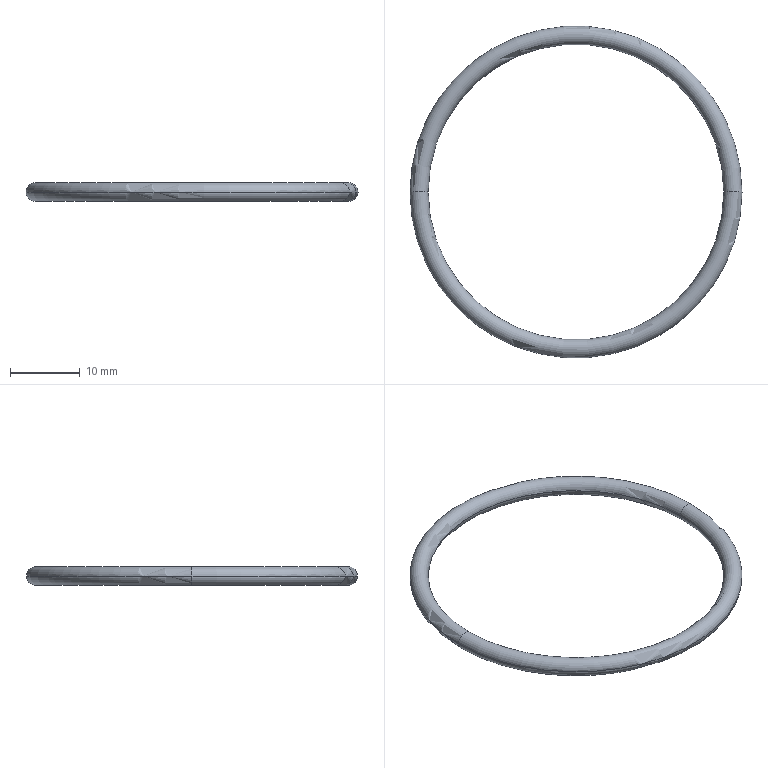Part | NX | features REVOLVE1 2 | 1 solid | 4 faces | box 47.752 x 47.752 x 2.616 mm | volume 762.259 mm3 | torus 4
STEP:
#1=CARTESIAN_POINT('',(-23.876,0.,0.));
#2=VERTEX_POINT('',#1);
#3=CARTESIAN_POINT('',(-21.26,0.,0.));
#4=VERTEX_POINT('',#3);
#5=CARTESIAN_POINT('',(-22.568,0.,0.));
#6=DIRECTION('',(0.,1.,0.));
#7=DIRECTION('',(-1.,0.,0.));
#8=AXIS2_PLACEMENT_3D('',#5,#6,#7);
#9=CIRCLE('',#8,1.308);
#10=EDGE_CURVE('',#2,#4,#9,.T.);
#11=ORIENTED_EDGE('',*,*,#10,.F.);
#12=CARTESIAN_POINT('',(23.876,0.,0.));
#13=VERTEX_POINT('',#12);
#14=CARTESIAN_POINT('',(0.,0.,0.));
#15=DIRECTION('',(0.,0.,1.));
#16=DIRECTION('',(1.,0.,0.));
#17=AXIS2_PLACEMENT_3D('',#14,#15,#16);
#18=CIRCLE('',#17,23.876);
#19=EDGE_CURVE('',#2,#13,#18,.T.);
#20=ORIENTED_EDGE('',*,*,#19,.T.);
#21=CARTESIAN_POINT('',(21.26,0.,0.));
#22=VERTEX_POINT('',#21);
#23=CARTESIAN_POINT('',(22.568,0.,0.));
#24=DIRECTION('',(0.,-1.,0.));
#25=DIRECTION('',(0.,0.,-1.));
#26=AXIS2_PLACEMENT_3D('',#23,#24,#25);
#27=CIRCLE('',#26,1.308);
#28=EDGE_CURVE('',#22,#13,#27,.F.);
#29=ORIENTED_EDGE('',*,*,#28,.F.);
#30=CARTESIAN_POINT('',(0.,0.,0.));
#31=DIRECTION('',(0.,0.,1.));
#32=DIRECTION('',(1.,0.,0.));
#33=AXIS2_PLACEMENT_3D('',#30,#31,#32);
#34=CIRCLE('',#33,21.26);
#35=EDGE_CURVE('',#22,#4,#34,.F.);
#36=ORIENTED_EDGE('',*,*,#35,.T.);
#37=EDGE_LOOP('',(#11,#20,#29,#36));
#38=FACE_BOUND('',#37,.T.);
#39=CARTESIAN_POINT('',(0.,0.,0.));
#40=DIRECTION('',(0.,0.,1.));
#41=DIRECTION('',(-1.,0.,0.));
#42=AXIS2_PLACEMENT_3D('',#39,#40,#41);
#43=TOROIDAL_SURFACE('',#42,22.568,1.308);
#44=ADVANCED_FACE('',(#38),#43,.T.);
#45=ORIENTED_EDGE('',*,*,#28,.T.);
#46=CARTESIAN_POINT('',(0.,0.,0.));
#47=DIRECTION('',(0.,0.,1.));
#48=DIRECTION('',(1.,0.,0.));
#49=AXIS2_PLACEMENT_3D('',#46,#47,#48);
#50=CIRCLE('',#49,23.876);
#51=EDGE_CURVE('',#13,#2,#50,.T.);
#52=ORIENTED_EDGE('',*,*,#51,.T.);
#53=ORIENTED_EDGE('',*,*,#10,.T.);
#54=CARTESIAN_POINT('',(0.,0.,0.));
#55=DIRECTION('',(0.,0.,1.));
#56=DIRECTION('',(1.,0.,0.));
#57=AXIS2_PLACEMENT_3D('',#54,#55,#56);
#58=CIRCLE('',#57,21.26);
#59=EDGE_CURVE('',#4,#22,#58,.F.);
#60=ORIENTED_EDGE('',*,*,#59,.T.);
#61=EDGE_LOOP('',(#45,#52,#53,#60));
#62=FACE_BOUND('',#61,.T.);
#63=CARTESIAN_POINT('',(0.,0.,0.));
#64=DIRECTION('',(0.,0.,1.));
#65=DIRECTION('',(-1.,0.,0.));
#66=AXIS2_PLACEMENT_3D('',#63,#64,#65);
#67=TOROIDAL_SURFACE('',#66,22.568,1.308);
#68=ADVANCED_FACE('',(#62),#67,.T.);
#69=ORIENTED_EDGE('',*,*,#51,.F.);
#70=CARTESIAN_POINT('',(22.568,0.,0.));
#71=DIRECTION('',(0.,-1.,0.));
#72=DIRECTION('',(0.,0.,-1.));
#73=AXIS2_PLACEMENT_3D('',#70,#71,#72);
#74=CIRCLE('',#73,1.308);
#75=EDGE_CURVE('',#22,#13,#74,.T.);
#76=ORIENTED_EDGE('',*,*,#75,.F.);
#77=ORIENTED_EDGE('',*,*,#59,.F.);
#78=CARTESIAN_POINT('',(-22.568,0.,0.));
#79=DIRECTION('',(0.,1.,0.));
#80=DIRECTION('',(-1.,0.,0.));
#81=AXIS2_PLACEMENT_3D('',#78,#79,#80);
#82=CIRCLE('',#81,1.308);
#83=EDGE_CURVE('',#2,#4,#82,.F.);
#84=ORIENTED_EDGE('',*,*,#83,.F.);
#85=EDGE_LOOP('',(#69,#76,#77,#84));
#86=FACE_BOUND('',#85,.T.);
#87=CARTESIAN_POINT('',(0.,0.,0.));
#88=DIRECTION('',(0.,0.,1.));
#89=DIRECTION('',(-1.,0.,0.));
#90=AXIS2_PLACEMENT_3D('',#87,#88,#89);
#91=TOROIDAL_SURFACE('',#90,22.568,1.308);
#92=ADVANCED_FACE('',(#86),#91,.T.);
#93=ORIENTED_EDGE('',*,*,#19,.F.);
#94=ORIENTED_EDGE('',*,*,#83,.T.);
#95=ORIENTED_EDGE('',*,*,#35,.F.);
#96=ORIENTED_EDGE('',*,*,#75,.T.);
#97=EDGE_LOOP('',(#93,#94,#95,#96));
#98=FACE_BOUND('',#97,.T.);
#99=CARTESIAN_POINT('',(0.,0.,0.));
#100=DIRECTION('',(0.,0.,1.));
#101=DIRECTION('',(-1.,0.,0.));
#102=AXIS2_PLACEMENT_3D('',#99,#100,#101);
#103=TOROIDAL_SURFACE('',#102,22.568,1.308);
#104=ADVANCED_FACE('',(#98),#103,.T.);
#105=CLOSED_SHELL('',(#44,#68,#92,#104));
#106=MANIFOLD_SOLID_BREP('',#105);
#107=(LENGTH_UNIT()NAMED_UNIT(*)SI_UNIT(.MILLI.,.METRE.));
#108=UNCERTAINTY_MEASURE_WITH_UNIT(LENGTH_MEASURE(0.00001),#107,'','');
#109=(NAMED_UNIT(*)PLANE_ANGLE_UNIT()SI_UNIT($,.RADIAN.));
#110=(NAMED_UNIT(*)SI_UNIT($,.STERADIAN.)SOLID_ANGLE_UNIT());
#111=(GEOMETRIC_REPRESENTATION_CONTEXT(3)GLOBAL_UNCERTAINTY_ASSIGNED_CONTEXT((#108))GLOBAL_UNIT_ASSIGNED_CONTEXT((#107,#109,#110))REPRESENTATION_CONTEXT('',''));
#112=ADVANCED_BREP_SHAPE_REPRESENTATION('',(#106),#111);